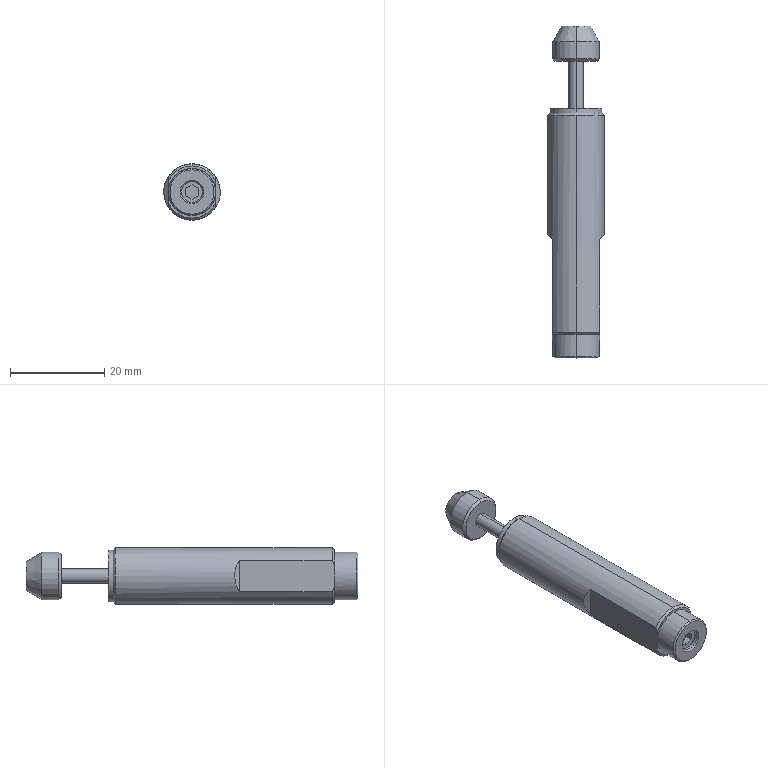Part | SolidWorks | features BaseBody 1 | 1 solid | 46 faces | box 12 x 70.5 x 12 mm | volume 6151 mm3 | plane 19 | cone 15 | cylinder 12 | commonest cylinder face diameters 10 x4 3 x2 4.459 x2 11 x2 12 x2
STEP:
#1=CARTESIAN_POINT('',(6.,51.54,0.));
#2=VERTEX_POINT('',#1);
#3=CARTESIAN_POINT('',(0.,51.54,6.));
#4=VERTEX_POINT('',#3);
#5=CARTESIAN_POINT('',(0.,51.54,0.));
#6=DIRECTION('',(0.,-1.,0.));
#7=DIRECTION('',(0.,0.,-1.));
#8=AXIS2_PLACEMENT_3D('',#5,#6,#7);
#9=CIRCLE('',#8,6.);
#10=EDGE_CURVE('',#2,#4,#9,.T.);
#11=ORIENTED_EDGE('',*,*,#10,.T.);
#12=CARTESIAN_POINT('',(0.,5.46,6.));
#13=VERTEX_POINT('',#12);
#14=CARTESIAN_POINT('',(0.,0.,6.));
#15=DIRECTION('',(0.,-1.,0.));
#16=VECTOR('',#15,1000.);
#17=LINE('',#14,#16);
#18=EDGE_CURVE('',#4,#13,#17,.T.);
#19=ORIENTED_EDGE('',*,*,#18,.T.);
#20=CARTESIAN_POINT('',(5.,5.46,3.317));
#21=VERTEX_POINT('',#20);
#22=CARTESIAN_POINT('',(0.,5.46,0.));
#23=DIRECTION('',(0.,1.,0.));
#24=DIRECTION('',(0.,0.,-1.));
#25=AXIS2_PLACEMENT_3D('',#22,#23,#24);
#26=CIRCLE('',#25,6.);
#27=EDGE_CURVE('',#13,#21,#26,.T.);
#28=ORIENTED_EDGE('',*,*,#27,.T.);
#29=CARTESIAN_POINT('',(5.,25.177,3.317));
#30=VERTEX_POINT('',#29);
#31=CARTESIAN_POINT('',(5.,0.,3.317));
#32=DIRECTION('',(0.,1.,0.));
#33=VECTOR('',#32,1000.);
#34=LINE('',#31,#33);
#35=EDGE_CURVE('',#21,#30,#34,.T.);
#36=ORIENTED_EDGE('',*,*,#35,.T.);
#37=CARTESIAN_POINT('',(5.,25.177,-3.317));
#38=VERTEX_POINT('',#37);
#39=CARTESIAN_POINT('',(5.,25.177,3.317));
#40=CARTESIAN_POINT('',(6.375,26.552,1.244));
#41=CARTESIAN_POINT('',(6.375,26.552,-1.244));
#42=CARTESIAN_POINT('',(5.,25.177,-3.317));
#43=(BOUNDED_CURVE()B_SPLINE_CURVE(3,(#39,#40,#41,#42),.UNSPECIFIED.,.F.,.F.)B_SPLINE_CURVE_WITH_KNOTS((4,4),(2.556,3.727),.UNSPECIFIED.)CURVE()GEOMETRIC_REPRESENTATION_ITEM()RATIONAL_B_SPLINE_CURVE((1.,0.8889,0.8889,1.))REPRESENTATION_ITEM(''));
#44=EDGE_CURVE('',#30,#38,#43,.T.);
#45=ORIENTED_EDGE('',*,*,#44,.T.);
#46=CARTESIAN_POINT('',(5.,5.46,-3.317));
#47=VERTEX_POINT('',#46);
#48=CARTESIAN_POINT('',(5.,0.,-3.317));
#49=DIRECTION('',(0.,-1.,0.));
#50=VECTOR('',#49,1000.);
#51=LINE('',#48,#50);
#52=EDGE_CURVE('',#38,#47,#51,.T.);
#53=ORIENTED_EDGE('',*,*,#52,.T.);
#54=CARTESIAN_POINT('',(0.,5.46,-6.));
#55=VERTEX_POINT('',#54);
#56=CARTESIAN_POINT('',(0.,5.46,0.));
#57=DIRECTION('',(0.,1.,0.));
#58=DIRECTION('',(0.,0.,-1.));
#59=AXIS2_PLACEMENT_3D('',#56,#57,#58);
#60=CIRCLE('',#59,6.);
#61=EDGE_CURVE('',#47,#55,#60,.T.);
#62=ORIENTED_EDGE('',*,*,#61,.T.);
#63=CARTESIAN_POINT('',(0.,51.54,-6.));
#64=VERTEX_POINT('',#63);
#65=CARTESIAN_POINT('',(0.,0.,-6.));
#66=DIRECTION('',(0.,-1.,0.));
#67=VECTOR('',#66,1000.);
#68=LINE('',#65,#67);
#69=EDGE_CURVE('',#64,#55,#68,.T.);
#70=ORIENTED_EDGE('',*,*,#69,.F.);
#71=CARTESIAN_POINT('',(0.,51.54,0.));
#72=DIRECTION('',(0.,-1.,0.));
#73=DIRECTION('',(0.,0.,-1.));
#74=AXIS2_PLACEMENT_3D('',#71,#72,#73);
#75=CIRCLE('',#74,6.);
#76=EDGE_CURVE('',#64,#2,#75,.T.);
#77=ORIENTED_EDGE('',*,*,#76,.T.);
#78=EDGE_LOOP('',(#11,#19,#28,#36,#45,#53,#62,#70,#77));
#79=FACE_OUTER_BOUND('',#78,.T.);
#80=CARTESIAN_POINT('',(0.,0.,0.));
#81=DIRECTION('',(0.,-1.,0.));
#82=DIRECTION('',(0.,0.,-1.));
#83=AXIS2_PLACEMENT_3D('',#80,#81,#82);
#84=CYLINDRICAL_SURFACE('',#83,6.);
#85=ADVANCED_FACE('',(#79),#84,.T.);
#86=CARTESIAN_POINT('',(5.54,52.,0.));
#87=VERTEX_POINT('',#86);
#88=CARTESIAN_POINT('',(-5.54,52.,0.));
#89=VERTEX_POINT('',#88);
#90=CARTESIAN_POINT('',(0.,52.,0.));
#91=DIRECTION('',(0.,-1.,0.));
#92=DIRECTION('',(1.,0.,0.));
#93=AXIS2_PLACEMENT_3D('',#90,#91,#92);
#94=CIRCLE('',#93,5.54);
#95=EDGE_CURVE('',#87,#89,#94,.T.);
#96=ORIENTED_EDGE('',*,*,#95,.T.);
#97=CARTESIAN_POINT('',(-6.,51.54,0.));
#98=VERTEX_POINT('',#97);
#99=CARTESIAN_POINT('',(-6.,51.54,0.));
#100=DIRECTION('',(-0.7071,-0.7071,0.));
#101=VECTOR('',#100,1000.);
#102=LINE('',#99,#101);
#103=EDGE_CURVE('',#89,#98,#102,.T.);
#104=ORIENTED_EDGE('',*,*,#103,.T.);
#105=CARTESIAN_POINT('',(0.,51.54,0.));
#106=DIRECTION('',(0.,-1.,0.));
#107=DIRECTION('',(0.,0.,-1.));
#108=AXIS2_PLACEMENT_3D('',#105,#106,#107);
#109=CIRCLE('',#108,6.);
#110=EDGE_CURVE('',#4,#98,#109,.T.);
#111=ORIENTED_EDGE('',*,*,#110,.F.);
#112=ORIENTED_EDGE('',*,*,#10,.F.);
#113=CARTESIAN_POINT('',(6.,51.54,0.));
#114=DIRECTION('',(0.7071,-0.7071,0.));
#115=VECTOR('',#114,1000.);
#116=LINE('',#113,#115);
#117=EDGE_CURVE('',#87,#2,#116,.T.);
#118=ORIENTED_EDGE('',*,*,#117,.F.);
#119=EDGE_LOOP('',(#96,#104,#111,#112,#118));
#120=FACE_OUTER_BOUND('',#119,.T.);
#121=CARTESIAN_POINT('',(0.,51.54,0.));
#122=DIRECTION('',(0.,-1.,0.));
#123=DIRECTION('',(1.,0.,0.));
#124=AXIS2_PLACEMENT_3D('',#121,#122,#123);
#125=CONICAL_SURFACE('',#124,6.,0.7854);
#126=ADVANCED_FACE('',(#120),#125,.T.);
#127=CARTESIAN_POINT('',(-5.,5.,2.386));
#128=VERTEX_POINT('',#127);
#129=CARTESIAN_POINT('',(0.,5.,5.54));
#130=VERTEX_POINT('',#129);
#131=CARTESIAN_POINT('',(0.,5.,0.));
#132=DIRECTION('',(0.,1.,0.));
#133=DIRECTION('',(0.,0.,1.));
#134=AXIS2_PLACEMENT_3D('',#131,#132,#133);
#135=CIRCLE('',#134,5.54);
#136=EDGE_CURVE('',#128,#130,#135,.T.);
#137=ORIENTED_EDGE('',*,*,#136,.T.);
#138=CARTESIAN_POINT('',(0.,5.46,6.));
#139=DIRECTION('',(0.,0.7071,0.7071));
#140=VECTOR('',#139,1000.);
#141=LINE('',#138,#140);
#142=EDGE_CURVE('',#130,#13,#141,.T.);
#143=ORIENTED_EDGE('',*,*,#142,.T.);
#144=CARTESIAN_POINT('',(-5.,5.46,3.317));
#145=VERTEX_POINT('',#144);
#146=CARTESIAN_POINT('',(0.,5.46,0.));
#147=DIRECTION('',(0.,1.,0.));
#148=DIRECTION('',(0.,0.,-1.));
#149=AXIS2_PLACEMENT_3D('',#146,#147,#148);
#150=CIRCLE('',#149,6.);
#151=EDGE_CURVE('',#145,#13,#150,.T.);
#152=ORIENTED_EDGE('',*,*,#151,.F.);
#153=CARTESIAN_POINT('',(-5.,5.46,3.317));
#154=CARTESIAN_POINT('',(-5.,5.292,3.013));
#155=CARTESIAN_POINT('',(-5.,5.137,2.704));
#156=CARTESIAN_POINT('',(-5.,5.,2.386));
#157=B_SPLINE_CURVE_WITH_KNOTS('',3,(#153,#154,#155,#156),.UNSPECIFIED.,.F.,.F.,(4,4),(0.,0.001038),.UNSPECIFIED.);
#158=EDGE_CURVE('',#145,#128,#157,.T.);
#159=ORIENTED_EDGE('',*,*,#158,.T.);
#160=EDGE_LOOP('',(#137,#143,#152,#159));
#161=FACE_OUTER_BOUND('',#160,.T.);
#162=CARTESIAN_POINT('',(0.,5.46,0.));
#163=DIRECTION('',(0.,1.,0.));
#164=DIRECTION('',(0.,0.,1.));
#165=AXIS2_PLACEMENT_3D('',#162,#163,#164);
#166=CONICAL_SURFACE('',#165,6.,0.7854);
#167=ADVANCED_FACE('',(#161),#166,.T.);
#168=CARTESIAN_POINT('',(0.,53.,-5.5));
#169=VERTEX_POINT('',#168);
#170=CARTESIAN_POINT('',(0.,53.,5.5));
#171=VERTEX_POINT('',#170);
#172=CARTESIAN_POINT('',(0.,53.,0.));
#173=DIRECTION('',(0.,-1.,0.));
#174=DIRECTION('',(0.,0.,-1.));
#175=AXIS2_PLACEMENT_3D('',#172,#173,#174);
#176=CIRCLE('',#175,5.5);
#177=EDGE_CURVE('',#169,#171,#176,.T.);
#178=ORIENTED_EDGE('',*,*,#177,.T.);
#179=CARTESIAN_POINT('',(0.,52.,5.5));
#180=VERTEX_POINT('',#179);
#181=CARTESIAN_POINT('',(0.,0.,5.5));
#182=DIRECTION('',(0.,-1.,0.));
#183=VECTOR('',#182,1000.);
#184=LINE('',#181,#183);
#185=EDGE_CURVE('',#171,#180,#184,.T.);
#186=ORIENTED_EDGE('',*,*,#185,.T.);
#187=CARTESIAN_POINT('',(0.,52.,-5.5));
#188=VERTEX_POINT('',#187);
#189=CARTESIAN_POINT('',(0.,52.,0.));
#190=DIRECTION('',(0.,1.,0.));
#191=DIRECTION('',(0.,0.,-1.));
#192=AXIS2_PLACEMENT_3D('',#189,#190,#191);
#193=CIRCLE('',#192,5.5);
#194=EDGE_CURVE('',#180,#188,#193,.T.);
#195=ORIENTED_EDGE('',*,*,#194,.T.);
#196=CARTESIAN_POINT('',(0.,0.,-5.5));
#197=DIRECTION('',(0.,-1.,0.));
#198=VECTOR('',#197,1000.);
#199=LINE('',#196,#198);
#200=EDGE_CURVE('',#169,#188,#199,.T.);
#201=ORIENTED_EDGE('',*,*,#200,.F.);
#202=EDGE_LOOP('',(#178,#186,#195,#201));
#203=FACE_OUTER_BOUND('',#202,.T.);
#204=CARTESIAN_POINT('',(0.,0.,0.));
#205=DIRECTION('',(0.,-1.,0.));
#206=DIRECTION('',(0.,0.,-1.));
#207=AXIS2_PLACEMENT_3D('',#204,#205,#206);
#208=CYLINDRICAL_SURFACE('',#207,5.5);
#209=ADVANCED_FACE('',(#203),#208,.T.);
#210=CARTESIAN_POINT('',(5.,5.,0.));
#211=VERTEX_POINT('',#210);
#212=CARTESIAN_POINT('',(0.,5.,5.));
#213=VERTEX_POINT('',#212);
#214=CARTESIAN_POINT('',(0.,5.,0.));
#215=DIRECTION('',(0.,-1.,0.));
#216=DIRECTION('',(0.,0.,-1.));
#217=AXIS2_PLACEMENT_3D('',#214,#215,#216);
#218=CIRCLE('',#217,5.);
#219=EDGE_CURVE('',#211,#213,#218,.T.);
#220=ORIENTED_EDGE('',*,*,#219,.T.);
#221=CARTESIAN_POINT('',(0.,0.3,5.));
#222=VERTEX_POINT('',#221);
#223=CARTESIAN_POINT('',(0.,0.,5.));
#224=DIRECTION('',(0.,-1.,0.));
#225=VECTOR('',#224,1000.);
#226=LINE('',#223,#225);
#227=EDGE_CURVE('',#213,#222,#226,.T.);
#228=ORIENTED_EDGE('',*,*,#227,.T.);
#229=CARTESIAN_POINT('',(0.,0.3,-5.));
#230=VERTEX_POINT('',#229);
#231=CARTESIAN_POINT('',(0.,0.3,0.));
#232=DIRECTION('',(0.,1.,0.));
#233=DIRECTION('',(0.,0.,-1.));
#234=AXIS2_PLACEMENT_3D('',#231,#232,#233);
#235=CIRCLE('',#234,5.);
#236=EDGE_CURVE('',#222,#230,#235,.T.);
#237=ORIENTED_EDGE('',*,*,#236,.T.);
#238=CARTESIAN_POINT('',(0.,5.,-5.));
#239=VERTEX_POINT('',#238);
#240=CARTESIAN_POINT('',(0.,0.,-5.));
#241=DIRECTION('',(0.,-1.,0.));
#242=VECTOR('',#241,1000.);
#243=LINE('',#240,#242);
#244=EDGE_CURVE('',#239,#230,#243,.T.);
#245=ORIENTED_EDGE('',*,*,#244,.F.);
#246=CARTESIAN_POINT('',(0.,5.,0.));
#247=DIRECTION('',(0.,-1.,0.));
#248=DIRECTION('',(0.,0.,-1.));
#249=AXIS2_PLACEMENT_3D('',#246,#247,#248);
#250=CIRCLE('',#249,5.);
#251=EDGE_CURVE('',#239,#211,#250,.T.);
#252=ORIENTED_EDGE('',*,*,#251,.T.);
#253=EDGE_LOOP('',(#220,#228,#237,#245,#252));
#254=FACE_OUTER_BOUND('',#253,.T.);
#255=CARTESIAN_POINT('',(0.,0.,0.));
#256=DIRECTION('',(0.,-1.,0.));
#257=DIRECTION('',(0.,0.,-1.));
#258=AXIS2_PLACEMENT_3D('',#255,#256,#257);
#259=CYLINDRICAL_SURFACE('',#258,5.);
#260=ADVANCED_FACE('',(#254),#259,.T.);
#261=CARTESIAN_POINT('',(0.,0.,4.7));
#262=VERTEX_POINT('',#261);
#263=CARTESIAN_POINT('',(0.,0.,-4.7));
#264=VERTEX_POINT('',#263);
#265=CARTESIAN_POINT('',(0.,0.,0.));
#266=DIRECTION('',(0.,1.,0.));
#267=DIRECTION('',(0.,0.,1.));
#268=AXIS2_PLACEMENT_3D('',#265,#266,#267);
#269=CIRCLE('',#268,4.7);
#270=EDGE_CURVE('',#262,#264,#269,.T.);
#271=ORIENTED_EDGE('',*,*,#270,.T.);
#272=CARTESIAN_POINT('',(0.,0.3,-5.));
#273=DIRECTION('',(0.,0.7071,-0.7071));
#274=VECTOR('',#273,1000.);
#275=LINE('',#272,#274);
#276=EDGE_CURVE('',#264,#230,#275,.T.);
#277=ORIENTED_EDGE('',*,*,#276,.T.);
#278=ORIENTED_EDGE('',*,*,#236,.F.);
#279=CARTESIAN_POINT('',(0.,0.3,5.));
#280=DIRECTION('',(0.,0.7071,0.7071));
#281=VECTOR('',#280,1000.);
#282=LINE('',#279,#281);
#283=EDGE_CURVE('',#262,#222,#282,.T.);
#284=ORIENTED_EDGE('',*,*,#283,.F.);
#285=EDGE_LOOP('',(#271,#277,#278,#284));
#286=FACE_OUTER_BOUND('',#285,.T.);
#287=CARTESIAN_POINT('',(0.,0.3,0.));
#288=DIRECTION('',(0.,1.,0.));
#289=DIRECTION('',(0.,0.,1.));
#290=AXIS2_PLACEMENT_3D('',#287,#288,#289);
#291=CONICAL_SURFACE('',#290,5.,0.7854);
#292=ADVANCED_FACE('',(#286),#291,.T.);
#293=CARTESIAN_POINT('',(0.,63.,-1.5));
#294=VERTEX_POINT('',#293);
#295=CARTESIAN_POINT('',(0.,63.,1.5));
#296=VERTEX_POINT('',#295);
#297=CARTESIAN_POINT('',(0.,63.,0.));
#298=DIRECTION('',(0.,-1.,0.));
#299=DIRECTION('',(0.,0.,-1.));
#300=AXIS2_PLACEMENT_3D('',#297,#298,#299);
#301=CIRCLE('',#300,1.5);
#302=EDGE_CURVE('',#294,#296,#301,.T.);
#303=ORIENTED_EDGE('',*,*,#302,.T.);
#304=CARTESIAN_POINT('',(0.,53.,1.5));
#305=VERTEX_POINT('',#304);
#306=CARTESIAN_POINT('',(0.,0.,1.5));
#307=DIRECTION('',(0.,-1.,0.));
#308=VECTOR('',#307,1000.);
#309=LINE('',#306,#308);
#310=EDGE_CURVE('',#296,#305,#309,.T.);
#311=ORIENTED_EDGE('',*,*,#310,.T.);
#312=CARTESIAN_POINT('',(0.,53.,-1.5));
#313=VERTEX_POINT('',#312);
#314=CARTESIAN_POINT('',(0.,53.,0.));
#315=DIRECTION('',(0.,1.,0.));
#316=DIRECTION('',(0.,0.,-1.));
#317=AXIS2_PLACEMENT_3D('',#314,#315,#316);
#318=CIRCLE('',#317,1.5);
#319=EDGE_CURVE('',#305,#313,#318,.T.);
#320=ORIENTED_EDGE('',*,*,#319,.T.);
#321=CARTESIAN_POINT('',(0.,0.,-1.5));
#322=DIRECTION('',(0.,-1.,0.));
#323=VECTOR('',#322,1000.);
#324=LINE('',#321,#323);
#325=EDGE_CURVE('',#294,#313,#324,.T.);
#326=ORIENTED_EDGE('',*,*,#325,.F.);
#327=EDGE_LOOP('',(#303,#311,#320,#326));
#328=FACE_OUTER_BOUND('',#327,.T.);
#329=CARTESIAN_POINT('',(0.,0.,0.));
#330=DIRECTION('',(0.,-1.,0.));
#331=DIRECTION('',(0.,0.,-1.));
#332=AXIS2_PLACEMENT_3D('',#329,#330,#331);
#333=CYLINDRICAL_SURFACE('',#332,1.5);
#334=ADVANCED_FACE('',(#328),#333,.T.);
#335=CARTESIAN_POINT('',(0.,0.2705,2.229));
#336=VERTEX_POINT('',#335);
#337=CARTESIAN_POINT('',(0.,0.2705,-2.229));
#338=VERTEX_POINT('',#337);
#339=CARTESIAN_POINT('',(0.,0.2705,0.));
#340=DIRECTION('',(0.,-1.,0.));
#341=DIRECTION('',(0.,0.,-1.));
#342=AXIS2_PLACEMENT_3D('',#339,#340,#341);
#343=CIRCLE('',#342,2.229);
#344=EDGE_CURVE('',#336,#338,#343,.T.);
#345=ORIENTED_EDGE('',*,*,#344,.F.);
#346=CARTESIAN_POINT('',(0.,0.,2.5));
#347=VERTEX_POINT('',#346);
#348=CARTESIAN_POINT('',(0.,0.,2.5));
#349=DIRECTION('',(0.,-0.7071,0.7071));
#350=VECTOR('',#349,1000.);
#351=LINE('',#348,#350);
#352=EDGE_CURVE('',#336,#347,#351,.T.);
#353=ORIENTED_EDGE('',*,*,#352,.T.);
#354=CARTESIAN_POINT('',(0.,0.,-2.5));
#355=VERTEX_POINT('',#354);
#356=CARTESIAN_POINT('',(0.,0.,0.));
#357=DIRECTION('',(0.,-1.,0.));
#358=DIRECTION('',(0.,0.,-1.));
#359=AXIS2_PLACEMENT_3D('',#356,#357,#358);
#360=CIRCLE('',#359,2.5);
#361=EDGE_CURVE('',#347,#355,#360,.T.);
#362=ORIENTED_EDGE('',*,*,#361,.T.);
#363=CARTESIAN_POINT('',(0.,0.,-2.5));
#364=DIRECTION('',(0.,-0.7071,-0.7071));
#365=VECTOR('',#364,1000.);
#366=LINE('',#363,#365);
#367=EDGE_CURVE('',#338,#355,#366,.T.);
#368=ORIENTED_EDGE('',*,*,#367,.F.);
#369=EDGE_LOOP('',(#345,#353,#362,#368));
#370=FACE_OUTER_BOUND('',#369,.T.);
#371=CARTESIAN_POINT('',(0.,0.,0.));
#372=DIRECTION('',(0.,-1.,0.));
#373=DIRECTION('',(0.,0.,-1.));
#374=AXIS2_PLACEMENT_3D('',#371,#372,#373);
#375=CONICAL_SURFACE('',#374,2.5,0.7854);
#376=ADVANCED_FACE('',(#370),#375,.F.);
#377=CARTESIAN_POINT('',(0.,63.,4.5));
#378=VERTEX_POINT('',#377);
#379=CARTESIAN_POINT('',(0.,63.,-4.5));
#380=VERTEX_POINT('',#379);
#381=CARTESIAN_POINT('',(0.,63.,0.));
#382=DIRECTION('',(0.,1.,0.));
#383=DIRECTION('',(0.,0.,1.));
#384=AXIS2_PLACEMENT_3D('',#381,#382,#383);
#385=CIRCLE('',#384,4.5);
#386=EDGE_CURVE('',#378,#380,#385,.T.);
#387=ORIENTED_EDGE('',*,*,#386,.T.);
#388=CARTESIAN_POINT('',(0.,63.5,-5.));
#389=VERTEX_POINT('',#388);
#390=CARTESIAN_POINT('',(0.,63.5,-5.));
#391=DIRECTION('',(0.,0.7071,-0.7071));
#392=VECTOR('',#391,1000.);
#393=LINE('',#390,#392);
#394=EDGE_CURVE('',#380,#389,#393,.T.);
#395=ORIENTED_EDGE('',*,*,#394,.T.);
#396=CARTESIAN_POINT('',(0.,63.5,5.));
#397=VERTEX_POINT('',#396);
#398=CARTESIAN_POINT('',(0.,63.5,0.));
#399=DIRECTION('',(0.,-1.,0.));
#400=DIRECTION('',(0.,0.,1.));
#401=AXIS2_PLACEMENT_3D('',#398,#399,#400);
#402=CIRCLE('',#401,5.);
#403=EDGE_CURVE('',#389,#397,#402,.T.);
#404=ORIENTED_EDGE('',*,*,#403,.T.);
#405=CARTESIAN_POINT('',(0.,63.5,5.));
#406=DIRECTION('',(0.,0.7071,0.7071));
#407=VECTOR('',#406,1000.);
#408=LINE('',#405,#407);
#409=EDGE_CURVE('',#378,#397,#408,.T.);
#410=ORIENTED_EDGE('',*,*,#409,.F.);
#411=EDGE_LOOP('',(#387,#395,#404,#410));
#412=FACE_OUTER_BOUND('',#411,.T.);
#413=CARTESIAN_POINT('',(0.,63.5,0.));
#414=DIRECTION('',(0.,1.,0.));
#415=DIRECTION('',(0.,0.,1.));
#416=AXIS2_PLACEMENT_3D('',#413,#414,#415);
#417=CONICAL_SURFACE('',#416,5.,0.7854);
#418=ADVANCED_FACE('',(#412),#417,.T.);
#419=CARTESIAN_POINT('',(0.,0.9295,2.229));
#420=VERTEX_POINT('',#419);
#421=CARTESIAN_POINT('',(0.,0.9295,-2.229));
#422=VERTEX_POINT('',#421);
#423=CARTESIAN_POINT('',(0.,0.9295,0.));
#424=DIRECTION('',(0.,-1.,0.));
#425=DIRECTION('',(0.,0.,-1.));
#426=AXIS2_PLACEMENT_3D('',#423,#424,#425);
#427=CIRCLE('',#426,2.229);
#428=EDGE_CURVE('',#420,#422,#427,.T.);
#429=ORIENTED_EDGE('',*,*,#428,.F.);
#430=CARTESIAN_POINT('',(0.,0.,2.229));
#431=DIRECTION('',(0.,-1.,0.));
#432=VECTOR('',#431,1000.);
#433=LINE('',#430,#432);
#434=EDGE_CURVE('',#420,#336,#433,.T.);
#435=ORIENTED_EDGE('',*,*,#434,.T.);
#436=ORIENTED_EDGE('',*,*,#344,.T.);
#437=CARTESIAN_POINT('',(0.,0.,-2.229));
#438=DIRECTION('',(0.,-1.,0.));
#439=VECTOR('',#438,1000.);
#440=LINE('',#437,#439);
#441=EDGE_CURVE('',#422,#338,#440,.T.);
#442=ORIENTED_EDGE('',*,*,#441,.F.);
#443=EDGE_LOOP('',(#429,#435,#436,#442));
#444=FACE_OUTER_BOUND('',#443,.T.);
#445=CARTESIAN_POINT('',(0.,0.,0.));
#446=DIRECTION('',(0.,-1.,0.));
#447=DIRECTION('',(0.,0.,-1.));
#448=AXIS2_PLACEMENT_3D('',#445,#446,#447);
#449=CYLINDRICAL_SURFACE('',#448,2.229);
#450=ADVANCED_FACE('',(#444),#449,.F.);
#451=CARTESIAN_POINT('',(0.,67.167,-5.));
#452=VERTEX_POINT('',#451);
#453=CARTESIAN_POINT('',(0.,67.167,5.));
#454=VERTEX_POINT('',#453);
#455=CARTESIAN_POINT('',(0.,67.167,0.));
#456=DIRECTION('',(0.,-1.,0.));
#457=DIRECTION('',(0.,0.,-1.));
#458=AXIS2_PLACEMENT_3D('',#455,#456,#457);
#459=CIRCLE('',#458,5.);
#460=EDGE_CURVE('',#452,#454,#459,.T.);
#461=ORIENTED_EDGE('',*,*,#460,.T.);
#462=CARTESIAN_POINT('',(0.,0.,5.));
#463=DIRECTION('',(0.,-1.,0.));
#464=VECTOR('',#463,1000.);
#465=LINE('',#462,#464);
#466=EDGE_CURVE('',#454,#397,#465,.T.);
#467=ORIENTED_EDGE('',*,*,#466,.T.);
#468=ORIENTED_EDGE('',*,*,#403,.F.);
#469=CARTESIAN_POINT('',(0.,0.,-5.));
#470=DIRECTION('',(0.,-1.,0.));
#471=VECTOR('',#470,1000.);
#472=LINE('',#469,#471);
#473=EDGE_CURVE('',#452,#389,#472,.T.);
#474=ORIENTED_EDGE('',*,*,#473,.F.);
#475=EDGE_LOOP('',(#461,#467,#468,#474));
#476=FACE_OUTER_BOUND('',#475,.T.);
#477=CARTESIAN_POINT('',(0.,0.,0.));
#478=DIRECTION('',(0.,-1.,0.));
#479=DIRECTION('',(0.,0.,-1.));
#480=AXIS2_PLACEMENT_3D('',#477,#478,#479);
#481=CYLINDRICAL_SURFACE('',#480,5.);
#482=ADVANCED_FACE('',(#476),#481,.T.);
#483=ORIENTED_EDGE('',*,*,#428,.T.);
#484=CARTESIAN_POINT('',(0.,1.2,-2.5));
#485=VERTEX_POINT('',#484);
#486=CARTESIAN_POINT('',(0.,1.2,-2.5));
#487=DIRECTION('',(0.,0.7071,-0.7071));
#488=VECTOR('',#487,1000.);
#489=LINE('',#486,#488);
#490=EDGE_CURVE('',#422,#485,#489,.T.);
#491=ORIENTED_EDGE('',*,*,#490,.T.);
#492=CARTESIAN_POINT('',(0.,1.2,2.5));
#493=VERTEX_POINT('',#492);
#494=CARTESIAN_POINT('',(0.,1.2,0.));
#495=DIRECTION('',(0.,-1.,0.));
#496=DIRECTION('',(0.,0.,1.));
#497=AXIS2_PLACEMENT_3D('',#494,#495,#496);
#498=CIRCLE('',#497,2.5);
#499=EDGE_CURVE('',#493,#485,#498,.T.);
#500=ORIENTED_EDGE('',*,*,#499,.F.);
#501=CARTESIAN_POINT('',(0.,1.2,2.5));
#502=DIRECTION('',(0.,0.7071,0.7071));
#503=VECTOR('',#502,1000.);
#504=LINE('',#501,#503);
#505=EDGE_CURVE('',#420,#493,#504,.T.);
#506=ORIENTED_EDGE('',*,*,#505,.F.);
#507=EDGE_LOOP('',(#483,#491,#500,#506));
#508=FACE_OUTER_BOUND('',#507,.T.);
#509=CARTESIAN_POINT('',(0.,1.2,0.));
#510=DIRECTION('',(0.,1.,0.));
#511=DIRECTION('',(0.,0.,1.));
#512=AXIS2_PLACEMENT_3D('',#509,#510,#511);
#513=CONICAL_SURFACE('',#512,2.5,0.7854);
#514=ADVANCED_FACE('',(#508),#513,.F.);
#515=CARTESIAN_POINT('',(0.,70.5,-3.075));
#516=VERTEX_POINT('',#515);
#517=CARTESIAN_POINT('',(0.,70.5,3.075));
#518=VERTEX_POINT('',#517);
#519=CARTESIAN_POINT('',(0.,70.5,0.));
#520=DIRECTION('',(0.,-1.,0.));
#521=DIRECTION('',(0.,0.,-1.));
#522=AXIS2_PLACEMENT_3D('',#519,#520,#521);
#523=CIRCLE('',#522,3.075);
#524=EDGE_CURVE('',#516,#518,#523,.T.);
#525=ORIENTED_EDGE('',*,*,#524,.T.);
#526=CARTESIAN_POINT('',(0.,67.167,5.));
#527=DIRECTION('',(0.,-0.866,0.5));
#528=VECTOR('',#527,1000.);
#529=LINE('',#526,#528);
#530=EDGE_CURVE('',#518,#454,#529,.T.);
#531=ORIENTED_EDGE('',*,*,#530,.T.);
#532=ORIENTED_EDGE('',*,*,#460,.F.);
#533=CARTESIAN_POINT('',(0.,67.167,-5.));
#534=DIRECTION('',(0.,-0.866,-0.5));
#535=VECTOR('',#534,1000.);
#536=LINE('',#533,#535);
#537=EDGE_CURVE('',#516,#452,#536,.T.);
#538=ORIENTED_EDGE('',*,*,#537,.F.);
#539=EDGE_LOOP('',(#525,#531,#532,#538));
#540=FACE_OUTER_BOUND('',#539,.T.);
#541=CARTESIAN_POINT('',(0.,67.167,0.));
#542=DIRECTION('',(0.,-1.,0.));
#543=DIRECTION('',(0.,0.,-1.));
#544=AXIS2_PLACEMENT_3D('',#541,#542,#543);
#545=CONICAL_SURFACE('',#544,5.,0.5236);
#546=ADVANCED_FACE('',(#540),#545,.T.);
#547=ORIENTED_EDGE('',*,*,#18,.F.);
#548=ORIENTED_EDGE('',*,*,#110,.T.);
#549=CARTESIAN_POINT('',(0.,51.54,0.));
#550=DIRECTION('',(0.,-1.,0.));
#551=DIRECTION('',(0.,0.,-1.));
#552=AXIS2_PLACEMENT_3D('',#549,#550,#551);
#553=CIRCLE('',#552,6.);
#554=EDGE_CURVE('',#98,#64,#553,.T.);
#555=ORIENTED_EDGE('',*,*,#554,.T.);
#556=ORIENTED_EDGE('',*,*,#69,.T.);
#557=CARTESIAN_POINT('',(-5.,5.46,-3.317));
#558=VERTEX_POINT('',#557);
#559=CARTESIAN_POINT('',(0.,5.46,0.));
#560=DIRECTION('',(0.,1.,0.));
#561=DIRECTION('',(0.,0.,-1.));
#562=AXIS2_PLACEMENT_3D('',#559,#560,#561);
#563=CIRCLE('',#562,6.);
#564=EDGE_CURVE('',#55,#558,#563,.T.);
#565=ORIENTED_EDGE('',*,*,#564,.T.);
#566=CARTESIAN_POINT('',(-5.,25.177,-3.317));
#567=VERTEX_POINT('',#566);
#568=CARTESIAN_POINT('',(-5.,0.,-3.317));
#569=DIRECTION('',(0.,1.,0.));
#570=VECTOR('',#569,1000.);
#571=LINE('',#568,#570);
#572=EDGE_CURVE('',#558,#567,#571,.T.);
#573=ORIENTED_EDGE('',*,*,#572,.T.);
#574=CARTESIAN_POINT('',(-5.,25.177,3.317));
#575=VERTEX_POINT('',#574);
#576=CARTESIAN_POINT('',(-5.,25.177,-3.317));
#577=CARTESIAN_POINT('',(-6.375,26.552,-1.244));
#578=CARTESIAN_POINT('',(-6.375,26.552,1.244));
#579=CARTESIAN_POINT('',(-5.,25.177,3.317));
#580=(BOUNDED_CURVE()B_SPLINE_CURVE(3,(#576,#577,#578,#579),.UNSPECIFIED.,.F.,.F.)B_SPLINE_CURVE_WITH_KNOTS((4,4),(2.556,3.727),.UNSPECIFIED.)CURVE()GEOMETRIC_REPRESENTATION_ITEM()RATIONAL_B_SPLINE_CURVE((1.,0.8889,0.8889,1.))REPRESENTATION_ITEM(''));
#581=EDGE_CURVE('',#567,#575,#580,.T.);
#582=ORIENTED_EDGE('',*,*,#581,.T.);
#583=CARTESIAN_POINT('',(-5.,0.,3.317));
#584=DIRECTION('',(0.,-1.,0.));
#585=VECTOR('',#584,1000.);
#586=LINE('',#583,#585);
#587=EDGE_CURVE('',#575,#145,#586,.T.);
#588=ORIENTED_EDGE('',*,*,#587,.T.);
#589=ORIENTED_EDGE('',*,*,#151,.T.);
#590=EDGE_LOOP('',(#547,#548,#555,#556,#565,#573,#582,#588,#589));
#591=FACE_OUTER_BOUND('',#590,.T.);
#592=CARTESIAN_POINT('',(0.,0.,0.));
#593=DIRECTION('',(0.,-1.,0.));
#594=DIRECTION('',(0.,0.,-1.));
#595=AXIS2_PLACEMENT_3D('',#592,#593,#594);
#596=CYLINDRICAL_SURFACE('',#595,6.);
#597=ADVANCED_FACE('',(#591),#596,.T.);
#598=ORIENTED_EDGE('',*,*,#103,.F.);
#599=CARTESIAN_POINT('',(0.,52.,0.));
#600=DIRECTION('',(0.,-1.,0.));
#601=DIRECTION('',(1.,0.,0.));
#602=AXIS2_PLACEMENT_3D('',#599,#600,#601);
#603=CIRCLE('',#602,5.54);
#604=EDGE_CURVE('',#89,#87,#603,.T.);
#605=ORIENTED_EDGE('',*,*,#604,.T.);
#606=ORIENTED_EDGE('',*,*,#117,.T.);
#607=ORIENTED_EDGE('',*,*,#76,.F.);
#608=ORIENTED_EDGE('',*,*,#554,.F.);
#609=EDGE_LOOP('',(#598,#605,#606,#607,#608));
#610=FACE_OUTER_BOUND('',#609,.T.);
#611=CARTESIAN_POINT('',(0.,51.54,0.));
#612=DIRECTION('',(0.,-1.,0.));
#613=DIRECTION('',(1.,0.,0.));
#614=AXIS2_PLACEMENT_3D('',#611,#612,#613);
#615=CONICAL_SURFACE('',#614,6.,0.7854);
#616=ADVANCED_FACE('',(#610),#615,.T.);
#617=ORIENTED_EDGE('',*,*,#142,.F.);
#618=CARTESIAN_POINT('',(5.,5.,2.386));
#619=VERTEX_POINT('',#618);
#620=CARTESIAN_POINT('',(0.,5.,0.));
#621=DIRECTION('',(0.,1.,0.));
#622=DIRECTION('',(0.,0.,1.));
#623=AXIS2_PLACEMENT_3D('',#620,#621,#622);
#624=CIRCLE('',#623,5.54);
#625=EDGE_CURVE('',#130,#619,#624,.T.);
#626=ORIENTED_EDGE('',*,*,#625,.T.);
#627=CARTESIAN_POINT('',(5.,5.,2.386));
#628=CARTESIAN_POINT('',(5.,5.137,2.704));
#629=CARTESIAN_POINT('',(5.,5.292,3.013));
#630=CARTESIAN_POINT('',(5.,5.46,3.317));
#631=B_SPLINE_CURVE_WITH_KNOTS('',3,(#627,#628,#629,#630),.UNSPECIFIED.,.F.,.F.,(4,4),(0.,0.001038),.UNSPECIFIED.);
#632=EDGE_CURVE('',#619,#21,#631,.T.);
#633=ORIENTED_EDGE('',*,*,#632,.T.);
#634=ORIENTED_EDGE('',*,*,#27,.F.);
#635=EDGE_LOOP('',(#617,#626,#633,#634));
#636=FACE_OUTER_BOUND('',#635,.T.);
#637=CARTESIAN_POINT('',(0.,5.46,0.));
#638=DIRECTION('',(0.,1.,0.));
#639=DIRECTION('',(0.,0.,1.));
#640=AXIS2_PLACEMENT_3D('',#637,#638,#639);
#641=CONICAL_SURFACE('',#640,6.,0.7854);
#642=ADVANCED_FACE('',(#636),#641,.T.);
#643=ORIENTED_EDGE('',*,*,#587,.F.);
#644=CARTESIAN_POINT('',(-5.,25.177,12.));
#645=DIRECTION('',(0.,0.,-1.));
#646=VECTOR('',#645,1000.);
#647=LINE('',#644,#646);
#648=EDGE_CURVE('',#575,#567,#647,.T.);
#649=ORIENTED_EDGE('',*,*,#648,.T.);
#650=ORIENTED_EDGE('',*,*,#572,.F.);
#651=CARTESIAN_POINT('',(-5.,5.,-2.386));
#652=VERTEX_POINT('',#651);
#653=CARTESIAN_POINT('',(-5.,5.46,-3.317));
#654=CARTESIAN_POINT('',(-5.,5.292,-3.013));
#655=CARTESIAN_POINT('',(-5.,5.137,-2.704));
#656=CARTESIAN_POINT('',(-5.,5.,-2.386));
#657=B_SPLINE_CURVE_WITH_KNOTS('',3,(#653,#654,#655,#656),.UNSPECIFIED.,.F.,.F.,(4,4),(0.,0.001038),.UNSPECIFIED.);
#658=EDGE_CURVE('',#558,#652,#657,.T.);
#659=ORIENTED_EDGE('',*,*,#658,.T.);
#660=CARTESIAN_POINT('',(-5.,5.,0.));
#661=VERTEX_POINT('',#660);
#662=CARTESIAN_POINT('',(-5.,5.,12.));
#663=DIRECTION('',(0.,0.,1.));
#664=VECTOR('',#663,1000.);
#665=LINE('',#662,#664);
#666=EDGE_CURVE('',#652,#661,#665,.T.);
#667=ORIENTED_EDGE('',*,*,#666,.T.);
#668=CARTESIAN_POINT('',(-5.,5.,12.));
#669=DIRECTION('',(0.,0.,1.));
#670=VECTOR('',#669,1000.);
#671=LINE('',#668,#670);
#672=EDGE_CURVE('',#661,#128,#671,.T.);
#673=ORIENTED_EDGE('',*,*,#672,.T.);
#674=ORIENTED_EDGE('',*,*,#158,.F.);
#675=EDGE_LOOP('',(#643,#649,#650,#659,#667,#673,#674));
#676=FACE_OUTER_BOUND('',#675,.T.);
#677=CARTESIAN_POINT('',(-5.,0.,12.));
#678=DIRECTION('',(-1.,0.,0.));
#679=DIRECTION('',(0.,-1.,0.));
#680=AXIS2_PLACEMENT_3D('',#677,#678,#679);
#681=PLANE('',#680);
#682=ADVANCED_FACE('',(#676),#681,.T.);
#683=ORIENTED_EDGE('',*,*,#581,.F.);
#684=ORIENTED_EDGE('',*,*,#648,.F.);
#685=EDGE_LOOP('',(#683,#684));
#686=FACE_OUTER_BOUND('',#685,.T.);
#687=CARTESIAN_POINT('',(-5.,25.177,12.));
#688=DIRECTION('',(-0.7071,-0.7071,0.));
#689=DIRECTION('',(0.7071,-0.7071,0.));
#690=AXIS2_PLACEMENT_3D('',#687,#688,#689);
#691=PLANE('',#690);
#692=ADVANCED_FACE('',(#686),#691,.T.);
#693=ORIENTED_EDGE('',*,*,#658,.F.);
#694=ORIENTED_EDGE('',*,*,#564,.F.);
#695=ORIENTED_EDGE('',*,*,#61,.F.);
#696=CARTESIAN_POINT('',(5.,5.,-2.386));
#697=VERTEX_POINT('',#696);
#698=CARTESIAN_POINT('',(5.,5.46,-3.317));
#699=CARTESIAN_POINT('',(5.,5.292,-3.013));
#700=CARTESIAN_POINT('',(5.,5.137,-2.704));
#701=CARTESIAN_POINT('',(5.,5.,-2.386));
#702=B_SPLINE_CURVE_WITH_KNOTS('',3,(#698,#699,#700,#701),.UNSPECIFIED.,.F.,.F.,(4,4),(0.,0.001038),.UNSPECIFIED.);
#703=EDGE_CURVE('',#47,#697,#702,.T.);
#704=ORIENTED_EDGE('',*,*,#703,.T.);
#705=CARTESIAN_POINT('',(0.,5.,0.));
#706=DIRECTION('',(0.,1.,0.));
#707=DIRECTION('',(0.,0.,1.));
#708=AXIS2_PLACEMENT_3D('',#705,#706,#707);
#709=CIRCLE('',#708,5.54);
#710=EDGE_CURVE('',#697,#652,#709,.T.);
#711=ORIENTED_EDGE('',*,*,#710,.T.);
#712=EDGE_LOOP('',(#693,#694,#695,#704,#711));
#713=FACE_OUTER_BOUND('',#712,.T.);
#714=CARTESIAN_POINT('',(0.,5.46,0.));
#715=DIRECTION('',(0.,1.,0.));
#716=DIRECTION('',(0.,0.,1.));
#717=AXIS2_PLACEMENT_3D('',#714,#715,#716);
#718=CONICAL_SURFACE('',#717,6.,0.7854);
#719=ADVANCED_FACE('',(#713),#718,.T.);
#720=ORIENTED_EDGE('',*,*,#52,.F.);
#721=CARTESIAN_POINT('',(5.,25.177,12.));
#722=DIRECTION('',(0.,0.,1.));
#723=VECTOR('',#722,1000.);
#724=LINE('',#721,#723);
#725=EDGE_CURVE('',#38,#30,#724,.T.);
#726=ORIENTED_EDGE('',*,*,#725,.T.);
#727=ORIENTED_EDGE('',*,*,#35,.F.);
#728=ORIENTED_EDGE('',*,*,#632,.F.);
#729=CARTESIAN_POINT('',(5.,5.,12.));
#730=DIRECTION('',(0.,0.,-1.));
#731=VECTOR('',#730,1000.);
#732=LINE('',#729,#731);
#733=EDGE_CURVE('',#619,#211,#732,.T.);
#734=ORIENTED_EDGE('',*,*,#733,.T.);
#735=CARTESIAN_POINT('',(5.,5.,12.));
#736=DIRECTION('',(0.,0.,-1.));
#737=VECTOR('',#736,1000.);
#738=LINE('',#735,#737);
#739=EDGE_CURVE('',#211,#697,#738,.T.);
#740=ORIENTED_EDGE('',*,*,#739,.T.);
#741=ORIENTED_EDGE('',*,*,#703,.F.);
#742=EDGE_LOOP('',(#720,#726,#727,#728,#734,#740,#741));
#743=FACE_OUTER_BOUND('',#742,.T.);
#744=CARTESIAN_POINT('',(5.,25.177,12.));
#745=DIRECTION('',(1.,0.,0.));
#746=DIRECTION('',(0.,1.,0.));
#747=AXIS2_PLACEMENT_3D('',#744,#745,#746);
#748=PLANE('',#747);
#749=ADVANCED_FACE('',(#743),#748,.T.);
#750=ORIENTED_EDGE('',*,*,#44,.F.);
#751=ORIENTED_EDGE('',*,*,#725,.F.);
#752=EDGE_LOOP('',(#750,#751));
#753=FACE_OUTER_BOUND('',#752,.T.);
#754=CARTESIAN_POINT('',(6.,26.177,12.));
#755=DIRECTION('',(0.7071,-0.7071,0.));
#756=DIRECTION('',(0.7071,0.7071,0.));
#757=AXIS2_PLACEMENT_3D('',#754,#755,#756);
#758=PLANE('',#757);
#759=ADVANCED_FACE('',(#753),#758,.T.);
#760=CARTESIAN_POINT('',(0.,52.,0.));
#761=DIRECTION('',(0.,1.,0.));
#762=DIRECTION('',(0.,0.,-1.));
#763=AXIS2_PLACEMENT_3D('',#760,#761,#762);
#764=CIRCLE('',#763,5.5);
#765=EDGE_CURVE('',#188,#180,#764,.T.);
#766=ORIENTED_EDGE('',*,*,#765,.F.);
#767=ORIENTED_EDGE('',*,*,#194,.F.);
#768=EDGE_LOOP('',(#766,#767));
#769=FACE_BOUND('',#768,.T.);
#770=ORIENTED_EDGE('',*,*,#95,.F.);
#771=ORIENTED_EDGE('',*,*,#604,.F.);
#772=EDGE_LOOP('',(#770,#771));
#773=FACE_OUTER_BOUND('',#772,.T.);
#774=CARTESIAN_POINT('',(5.5,52.,0.));
#775=DIRECTION('',(0.,-1.,0.));
#776=DIRECTION('',(0.,0.,-1.));
#777=AXIS2_PLACEMENT_3D('',#774,#775,#776);
#778=PLANE('',#777);
#779=ADVANCED_FACE('',(#769,#773),#778,.F.);
#780=ORIENTED_EDGE('',*,*,#136,.F.);
#781=ORIENTED_EDGE('',*,*,#672,.F.);
#782=CARTESIAN_POINT('',(0.,5.,0.));
#783=DIRECTION('',(0.,-1.,0.));
#784=DIRECTION('',(0.,0.,-1.));
#785=AXIS2_PLACEMENT_3D('',#782,#783,#784);
#786=CIRCLE('',#785,5.);
#787=EDGE_CURVE('',#213,#661,#786,.T.);
#788=ORIENTED_EDGE('',*,*,#787,.F.);
#789=ORIENTED_EDGE('',*,*,#219,.F.);
#790=ORIENTED_EDGE('',*,*,#733,.F.);
#791=ORIENTED_EDGE('',*,*,#625,.F.);
#792=EDGE_LOOP('',(#780,#781,#788,#789,#790,#791));
#793=FACE_OUTER_BOUND('',#792,.T.);
#794=CARTESIAN_POINT('',(5.54,5.,0.));
#795=DIRECTION('',(0.,1.,0.));
#796=DIRECTION('',(0.,0.,1.));
#797=AXIS2_PLACEMENT_3D('',#794,#795,#796);
#798=PLANE('',#797);
#799=ADVANCED_FACE('',(#793),#798,.F.);
#800=CARTESIAN_POINT('',(0.,5.,0.));
#801=DIRECTION('',(0.,-1.,0.));
#802=DIRECTION('',(0.,0.,-1.));
#803=AXIS2_PLACEMENT_3D('',#800,#801,#802);
#804=CIRCLE('',#803,5.);
#805=EDGE_CURVE('',#661,#239,#804,.T.);
#806=ORIENTED_EDGE('',*,*,#805,.F.);
#807=ORIENTED_EDGE('',*,*,#666,.F.);
#808=ORIENTED_EDGE('',*,*,#710,.F.);
#809=ORIENTED_EDGE('',*,*,#739,.F.);
#810=ORIENTED_EDGE('',*,*,#251,.F.);
#811=EDGE_LOOP('',(#806,#807,#808,#809,#810));
#812=FACE_OUTER_BOUND('',#811,.T.);
#813=CARTESIAN_POINT('',(5.54,5.,0.));
#814=DIRECTION('',(0.,1.,0.));
#815=DIRECTION('',(0.,0.,1.));
#816=AXIS2_PLACEMENT_3D('',#813,#814,#815);
#817=PLANE('',#816);
#818=ADVANCED_FACE('',(#812),#817,.F.);
#819=ORIENTED_EDGE('',*,*,#185,.F.);
#820=CARTESIAN_POINT('',(0.,53.,0.));
#821=DIRECTION('',(0.,-1.,0.));
#822=DIRECTION('',(0.,0.,-1.));
#823=AXIS2_PLACEMENT_3D('',#820,#821,#822);
#824=CIRCLE('',#823,5.5);
#825=EDGE_CURVE('',#171,#169,#824,.T.);
#826=ORIENTED_EDGE('',*,*,#825,.T.);
#827=ORIENTED_EDGE('',*,*,#200,.T.);
#828=ORIENTED_EDGE('',*,*,#765,.T.);
#829=EDGE_LOOP('',(#819,#826,#827,#828));
#830=FACE_OUTER_BOUND('',#829,.T.);
#831=CARTESIAN_POINT('',(0.,0.,0.));
#832=DIRECTION('',(0.,-1.,0.));
#833=DIRECTION('',(0.,0.,-1.));
#834=AXIS2_PLACEMENT_3D('',#831,#832,#833);
#835=CYLINDRICAL_SURFACE('',#834,5.5);
#836=ADVANCED_FACE('',(#830),#835,.T.);
#837=ORIENTED_EDGE('',*,*,#227,.F.);
#838=ORIENTED_EDGE('',*,*,#787,.T.);
#839=ORIENTED_EDGE('',*,*,#805,.T.);
#840=ORIENTED_EDGE('',*,*,#244,.T.);
#841=CARTESIAN_POINT('',(0.,0.3,0.));
#842=DIRECTION('',(0.,1.,0.));
#843=DIRECTION('',(0.,0.,-1.));
#844=AXIS2_PLACEMENT_3D('',#841,#842,#843);
#845=CIRCLE('',#844,5.);
#846=EDGE_CURVE('',#230,#222,#845,.T.);
#847=ORIENTED_EDGE('',*,*,#846,.T.);
#848=EDGE_LOOP('',(#837,#838,#839,#840,#847));
#849=FACE_OUTER_BOUND('',#848,.T.);
#850=CARTESIAN_POINT('',(0.,0.,0.));
#851=DIRECTION('',(0.,-1.,0.));
#852=DIRECTION('',(0.,0.,-1.));
#853=AXIS2_PLACEMENT_3D('',#850,#851,#852);
#854=CYLINDRICAL_SURFACE('',#853,5.);
#855=ADVANCED_FACE('',(#849),#854,.T.);
#856=CARTESIAN_POINT('',(0.,53.,0.));
#857=DIRECTION('',(0.,1.,0.));
#858=DIRECTION('',(0.,0.,-1.));
#859=AXIS2_PLACEMENT_3D('',#856,#857,#858);
#860=CIRCLE('',#859,1.5);
#861=EDGE_CURVE('',#313,#305,#860,.T.);
#862=ORIENTED_EDGE('',*,*,#861,.F.);
#863=ORIENTED_EDGE('',*,*,#319,.F.);
#864=EDGE_LOOP('',(#862,#863));
#865=FACE_BOUND('',#864,.T.);
#866=ORIENTED_EDGE('',*,*,#177,.F.);
#867=ORIENTED_EDGE('',*,*,#825,.F.);
#868=EDGE_LOOP('',(#866,#867));
#869=FACE_OUTER_BOUND('',#868,.T.);
#870=CARTESIAN_POINT('',(1.5,53.,0.));
#871=DIRECTION('',(0.,-1.,0.));
#872=DIRECTION('',(0.,0.,-1.));
#873=AXIS2_PLACEMENT_3D('',#870,#871,#872);
#874=PLANE('',#873);
#875=ADVANCED_FACE('',(#865,#869),#874,.F.);
#876=ORIENTED_EDGE('',*,*,#276,.F.);
#877=CARTESIAN_POINT('',(0.,0.,0.));
#878=DIRECTION('',(0.,1.,0.));
#879=DIRECTION('',(0.,0.,1.));
#880=AXIS2_PLACEMENT_3D('',#877,#878,#879);
#881=CIRCLE('',#880,4.7);
#882=EDGE_CURVE('',#264,#262,#881,.T.);
#883=ORIENTED_EDGE('',*,*,#882,.T.);
#884=ORIENTED_EDGE('',*,*,#283,.T.);
#885=ORIENTED_EDGE('',*,*,#846,.F.);
#886=EDGE_LOOP('',(#876,#883,#884,#885));
#887=FACE_OUTER_BOUND('',#886,.T.);
#888=CARTESIAN_POINT('',(0.,0.3,0.));
#889=DIRECTION('',(0.,1.,0.));
#890=DIRECTION('',(0.,0.,1.));
#891=AXIS2_PLACEMENT_3D('',#888,#889,#890);
#892=CONICAL_SURFACE('',#891,5.,0.7854);
#893=ADVANCED_FACE('',(#887),#892,.T.);
#894=ORIENTED_EDGE('',*,*,#310,.F.);
#895=CARTESIAN_POINT('',(0.,63.,0.));
#896=DIRECTION('',(0.,-1.,0.));
#897=DIRECTION('',(0.,0.,-1.));
#898=AXIS2_PLACEMENT_3D('',#895,#896,#897);
#899=CIRCLE('',#898,1.5);
#900=EDGE_CURVE('',#296,#294,#899,.T.);
#901=ORIENTED_EDGE('',*,*,#900,.T.);
#902=ORIENTED_EDGE('',*,*,#325,.T.);
#903=ORIENTED_EDGE('',*,*,#861,.T.);
#904=EDGE_LOOP('',(#894,#901,#902,#903));
#905=FACE_OUTER_BOUND('',#904,.T.);
#906=CARTESIAN_POINT('',(0.,0.,0.));
#907=DIRECTION('',(0.,-1.,0.));
#908=DIRECTION('',(0.,0.,-1.));
#909=AXIS2_PLACEMENT_3D('',#906,#907,#908);
#910=CYLINDRICAL_SURFACE('',#909,1.5);
#911=ADVANCED_FACE('',(#905),#910,.T.);
#912=ORIENTED_EDGE('',*,*,#270,.F.);
#913=ORIENTED_EDGE('',*,*,#882,.F.);
#914=EDGE_LOOP('',(#912,#913));
#915=FACE_OUTER_BOUND('',#914,.T.);
#916=CARTESIAN_POINT('',(0.,0.,0.));
#917=DIRECTION('',(0.,-1.,0.));
#918=DIRECTION('',(0.,0.,-1.));
#919=AXIS2_PLACEMENT_3D('',#916,#917,#918);
#920=CIRCLE('',#919,2.5);
#921=EDGE_CURVE('',#355,#347,#920,.T.);
#922=ORIENTED_EDGE('',*,*,#921,.F.);
#923=ORIENTED_EDGE('',*,*,#361,.F.);
#924=EDGE_LOOP('',(#922,#923));
#925=FACE_BOUND('',#924,.T.);
#926=CARTESIAN_POINT('',(4.7,0.,0.));
#927=DIRECTION('',(0.,1.,0.));
#928=DIRECTION('',(0.,0.,1.));
#929=AXIS2_PLACEMENT_3D('',#926,#927,#928);
#930=PLANE('',#929);
#931=ADVANCED_FACE('',(#915,#925),#930,.F.);
#932=ORIENTED_EDGE('',*,*,#386,.F.);
#933=CARTESIAN_POINT('',(0.,63.,0.));
#934=DIRECTION('',(0.,1.,0.));
#935=DIRECTION('',(0.,0.,1.));
#936=AXIS2_PLACEMENT_3D('',#933,#934,#935);
#937=CIRCLE('',#936,4.5);
#938=EDGE_CURVE('',#380,#378,#937,.T.);
#939=ORIENTED_EDGE('',*,*,#938,.F.);
#940=EDGE_LOOP('',(#932,#939));
#941=FACE_OUTER_BOUND('',#940,.T.);
#942=ORIENTED_EDGE('',*,*,#302,.F.);
#943=ORIENTED_EDGE('',*,*,#900,.F.);
#944=EDGE_LOOP('',(#942,#943));
#945=FACE_BOUND('',#944,.T.);
#946=CARTESIAN_POINT('',(4.5,63.,0.));
#947=DIRECTION('',(0.,1.,0.));
#948=DIRECTION('',(0.,0.,1.));
#949=AXIS2_PLACEMENT_3D('',#946,#947,#948);
#950=PLANE('',#949);
#951=ADVANCED_FACE('',(#941,#945),#950,.F.);
#952=ORIENTED_EDGE('',*,*,#352,.F.);
#953=CARTESIAN_POINT('',(0.,0.2705,0.));
#954=DIRECTION('',(0.,-1.,0.));
#955=DIRECTION('',(0.,0.,-1.));
#956=AXIS2_PLACEMENT_3D('',#953,#954,#955);
#957=CIRCLE('',#956,2.229);
#958=EDGE_CURVE('',#338,#336,#957,.T.);
#959=ORIENTED_EDGE('',*,*,#958,.F.);
#960=ORIENTED_EDGE('',*,*,#367,.T.);
#961=ORIENTED_EDGE('',*,*,#921,.T.);
#962=EDGE_LOOP('',(#952,#959,#960,#961));
#963=FACE_OUTER_BOUND('',#962,.T.);
#964=CARTESIAN_POINT('',(0.,0.,0.));
#965=DIRECTION('',(0.,-1.,0.));
#966=DIRECTION('',(0.,0.,-1.));
#967=AXIS2_PLACEMENT_3D('',#964,#965,#966);
#968=CONICAL_SURFACE('',#967,2.5,0.7854);
#969=ADVANCED_FACE('',(#963),#968,.F.);
#970=ORIENTED_EDGE('',*,*,#394,.F.);
#971=ORIENTED_EDGE('',*,*,#938,.T.);
#972=ORIENTED_EDGE('',*,*,#409,.T.);
#973=CARTESIAN_POINT('',(0.,63.5,0.));
#974=DIRECTION('',(0.,-1.,0.));
#975=DIRECTION('',(0.,0.,1.));
#976=AXIS2_PLACEMENT_3D('',#973,#974,#975);
#977=CIRCLE('',#976,5.);
#978=EDGE_CURVE('',#397,#389,#977,.T.);
#979=ORIENTED_EDGE('',*,*,#978,.T.);
#980=EDGE_LOOP('',(#970,#971,#972,#979));
#981=FACE_OUTER_BOUND('',#980,.T.);
#982=CARTESIAN_POINT('',(0.,63.5,0.));
#983=DIRECTION('',(0.,1.,0.));
#984=DIRECTION('',(0.,0.,1.));
#985=AXIS2_PLACEMENT_3D('',#982,#983,#984);
#986=CONICAL_SURFACE('',#985,5.,0.7854);
#987=ADVANCED_FACE('',(#981),#986,.T.);
#988=ORIENTED_EDGE('',*,*,#434,.F.);
#989=CARTESIAN_POINT('',(0.,0.9295,0.));
#990=DIRECTION('',(0.,-1.,0.));
#991=DIRECTION('',(0.,0.,-1.));
#992=AXIS2_PLACEMENT_3D('',#989,#990,#991);
#993=CIRCLE('',#992,2.229);
#994=EDGE_CURVE('',#422,#420,#993,.T.);
#995=ORIENTED_EDGE('',*,*,#994,.F.);
#996=ORIENTED_EDGE('',*,*,#441,.T.);
#997=ORIENTED_EDGE('',*,*,#958,.T.);
#998=EDGE_LOOP('',(#988,#995,#996,#997));
#999=FACE_OUTER_BOUND('',#998,.T.);
#1000=CARTESIAN_POINT('',(0.,0.,0.));
#1001=DIRECTION('',(0.,-1.,0.));
#1002=DIRECTION('',(0.,0.,-1.));
#1003=AXIS2_PLACEMENT_3D('',#1000,#1001,#1002);
#1004=CYLINDRICAL_SURFACE('',#1003,2.229);
#1005=ADVANCED_FACE('',(#999),#1004,.F.);
#1006=ORIENTED_EDGE('',*,*,#466,.F.);
#1007=CARTESIAN_POINT('',(0.,67.167,0.));
#1008=DIRECTION('',(0.,-1.,0.));
#1009=DIRECTION('',(0.,0.,-1.));
#1010=AXIS2_PLACEMENT_3D('',#1007,#1008,#1009);
#1011=CIRCLE('',#1010,5.);
#1012=EDGE_CURVE('',#454,#452,#1011,.T.);
#1013=ORIENTED_EDGE('',*,*,#1012,.T.);
#1014=ORIENTED_EDGE('',*,*,#473,.T.);
#1015=ORIENTED_EDGE('',*,*,#978,.F.);
#1016=EDGE_LOOP('',(#1006,#1013,#1014,#1015));
#1017=FACE_OUTER_BOUND('',#1016,.T.);
#1018=CARTESIAN_POINT('',(0.,0.,0.));
#1019=DIRECTION('',(0.,-1.,0.));
#1020=DIRECTION('',(0.,0.,-1.));
#1021=AXIS2_PLACEMENT_3D('',#1018,#1019,#1020);
#1022=CYLINDRICAL_SURFACE('',#1021,5.);
#1023=ADVANCED_FACE('',(#1017),#1022,.T.);
#1024=ORIENTED_EDGE('',*,*,#490,.F.);
#1025=ORIENTED_EDGE('',*,*,#994,.T.);
#1026=ORIENTED_EDGE('',*,*,#505,.T.);
#1027=CARTESIAN_POINT('',(0.,1.2,0.));
#1028=DIRECTION('',(0.,-1.,0.));
#1029=DIRECTION('',(0.,0.,1.));
#1030=AXIS2_PLACEMENT_3D('',#1027,#1028,#1029);
#1031=CIRCLE('',#1030,2.5);
#1032=EDGE_CURVE('',#485,#493,#1031,.T.);
#1033=ORIENTED_EDGE('',*,*,#1032,.F.);
#1034=EDGE_LOOP('',(#1024,#1025,#1026,#1033));
#1035=FACE_OUTER_BOUND('',#1034,.T.);
#1036=CARTESIAN_POINT('',(0.,1.2,0.));
#1037=DIRECTION('',(0.,1.,0.));
#1038=DIRECTION('',(0.,0.,1.));
#1039=AXIS2_PLACEMENT_3D('',#1036,#1037,#1038);
#1040=CONICAL_SURFACE('',#1039,2.5,0.7854);
#1041=ADVANCED_FACE('',(#1035),#1040,.F.);
#1042=ORIENTED_EDGE('',*,*,#530,.F.);
#1043=CARTESIAN_POINT('',(0.,70.5,0.));
#1044=DIRECTION('',(0.,-1.,0.));
#1045=DIRECTION('',(0.,0.,-1.));
#1046=AXIS2_PLACEMENT_3D('',#1043,#1044,#1045);
#1047=CIRCLE('',#1046,3.075);
#1048=EDGE_CURVE('',#518,#516,#1047,.T.);
#1049=ORIENTED_EDGE('',*,*,#1048,.T.);
#1050=ORIENTED_EDGE('',*,*,#537,.T.);
#1051=ORIENTED_EDGE('',*,*,#1012,.F.);
#1052=EDGE_LOOP('',(#1042,#1049,#1050,#1051));
#1053=FACE_OUTER_BOUND('',#1052,.T.);
#1054=CARTESIAN_POINT('',(0.,67.167,0.));
#1055=DIRECTION('',(0.,-1.,0.));
#1056=DIRECTION('',(0.,0.,-1.));
#1057=AXIS2_PLACEMENT_3D('',#1054,#1055,#1056);
#1058=CONICAL_SURFACE('',#1057,5.,0.5236);
#1059=ADVANCED_FACE('',(#1053),#1058,.T.);
#1060=CARTESIAN_POINT('',(1.299,1.2,0.75));
#1061=VERTEX_POINT('',#1060);
#1062=CARTESIAN_POINT('',(1.299,1.2,-0.75));
#1063=VERTEX_POINT('',#1062);
#1064=CARTESIAN_POINT('',(1.299,1.2,0.));
#1065=DIRECTION('',(0.,0.,-1.));
#1066=VECTOR('',#1065,1000.);
#1067=LINE('',#1064,#1066);
#1068=EDGE_CURVE('',#1061,#1063,#1067,.T.);
#1069=ORIENTED_EDGE('',*,*,#1068,.T.);
#1070=CARTESIAN_POINT('',(0.,1.2,-1.5));
#1071=VERTEX_POINT('',#1070);
#1072=CARTESIAN_POINT('',(1.299,1.2,-0.75));
#1073=DIRECTION('',(-0.866,0.,-0.5));
#1074=VECTOR('',#1073,1000.);
#1075=LINE('',#1072,#1074);
#1076=EDGE_CURVE('',#1063,#1071,#1075,.T.);
#1077=ORIENTED_EDGE('',*,*,#1076,.T.);
#1078=CARTESIAN_POINT('',(-1.299,1.2,-0.75));
#1079=VERTEX_POINT('',#1078);
#1080=CARTESIAN_POINT('',(0.,1.2,-1.5));
#1081=DIRECTION('',(-0.866,0.,0.5));
#1082=VECTOR('',#1081,1000.);
#1083=LINE('',#1080,#1082);
#1084=EDGE_CURVE('',#1071,#1079,#1083,.T.);
#1085=ORIENTED_EDGE('',*,*,#1084,.T.);
#1086=CARTESIAN_POINT('',(-1.299,1.2,0.75));
#1087=VERTEX_POINT('',#1086);
#1088=CARTESIAN_POINT('',(-1.299,1.2,0.));
#1089=DIRECTION('',(0.,0.,1.));
#1090=VECTOR('',#1089,1000.);
#1091=LINE('',#1088,#1090);
#1092=EDGE_CURVE('',#1079,#1087,#1091,.T.);
#1093=ORIENTED_EDGE('',*,*,#1092,.T.);
#1094=CARTESIAN_POINT('',(0.,1.2,1.5));
#1095=VERTEX_POINT('',#1094);
#1096=CARTESIAN_POINT('',(-1.299,1.2,0.75));
#1097=DIRECTION('',(0.866,0.,0.5));
#1098=VECTOR('',#1097,1000.);
#1099=LINE('',#1096,#1098);
#1100=EDGE_CURVE('',#1087,#1095,#1099,.T.);
#1101=ORIENTED_EDGE('',*,*,#1100,.T.);
#1102=CARTESIAN_POINT('',(0.,1.2,1.5));
#1103=DIRECTION('',(0.866,0.,-0.5));
#1104=VECTOR('',#1103,1000.);
#1105=LINE('',#1102,#1104);
#1106=EDGE_CURVE('',#1095,#1061,#1105,.T.);
#1107=ORIENTED_EDGE('',*,*,#1106,.T.);
#1108=EDGE_LOOP('',(#1069,#1077,#1085,#1093,#1101,#1107));
#1109=FACE_BOUND('',#1108,.T.);
#1110=ORIENTED_EDGE('',*,*,#499,.T.);
#1111=ORIENTED_EDGE('',*,*,#1032,.T.);
#1112=EDGE_LOOP('',(#1110,#1111));
#1113=FACE_OUTER_BOUND('',#1112,.T.);
#1114=CARTESIAN_POINT('',(0.,1.2,0.));
#1115=DIRECTION('',(0.,-1.,0.));
#1116=DIRECTION('',(0.,0.,-1.));
#1117=AXIS2_PLACEMENT_3D('',#1114,#1115,#1116);
#1118=PLANE('',#1117);
#1119=ADVANCED_FACE('',(#1109,#1113),#1118,.T.);
#1120=ORIENTED_EDGE('',*,*,#524,.F.);
#1121=ORIENTED_EDGE('',*,*,#1048,.F.);
#1122=EDGE_LOOP('',(#1120,#1121));
#1123=FACE_OUTER_BOUND('',#1122,.T.);
#1124=CARTESIAN_POINT('',(0.,70.5,0.));
#1125=DIRECTION('',(0.,-1.,0.));
#1126=DIRECTION('',(0.,0.,-1.));
#1127=AXIS2_PLACEMENT_3D('',#1124,#1125,#1126);
#1128=PLANE('',#1127);
#1129=ADVANCED_FACE('',(#1123),#1128,.F.);
#1130=CARTESIAN_POINT('',(0.,2.5,-1.5));
#1131=VERTEX_POINT('',#1130);
#1132=CARTESIAN_POINT('',(0.,2.5,-1.5));
#1133=DIRECTION('',(0.,-1.,0.));
#1134=VECTOR('',#1133,1000.);
#1135=LINE('',#1132,#1134);
#1136=EDGE_CURVE('',#1131,#1071,#1135,.T.);
#1137=ORIENTED_EDGE('',*,*,#1136,.T.);
#1138=ORIENTED_EDGE('',*,*,#1076,.F.);
#1139=CARTESIAN_POINT('',(1.299,2.5,-0.75));
#1140=VERTEX_POINT('',#1139);
#1141=CARTESIAN_POINT('',(1.299,2.5,-0.75));
#1142=DIRECTION('',(0.,1.,0.));
#1143=VECTOR('',#1142,1000.);
#1144=LINE('',#1141,#1143);
#1145=EDGE_CURVE('',#1063,#1140,#1144,.T.);
#1146=ORIENTED_EDGE('',*,*,#1145,.T.);
#1147=CARTESIAN_POINT('',(1.299,2.5,-0.75));
#1148=DIRECTION('',(-0.866,0.,-0.5));
#1149=VECTOR('',#1148,1000.);
#1150=LINE('',#1147,#1149);
#1151=EDGE_CURVE('',#1140,#1131,#1150,.T.);
#1152=ORIENTED_EDGE('',*,*,#1151,.T.);
#1153=EDGE_LOOP('',(#1137,#1138,#1146,#1152));
#1154=FACE_OUTER_BOUND('',#1153,.T.);
#1155=CARTESIAN_POINT('',(1.299,2.5,-0.75));
#1156=DIRECTION('',(-0.5,0.,0.866));
#1157=DIRECTION('',(0.866,0.,0.5));
#1158=AXIS2_PLACEMENT_3D('',#1155,#1156,#1157);
#1159=PLANE('',#1158);
#1160=ADVANCED_FACE('',(#1154),#1159,.T.);
#1161=ORIENTED_EDGE('',*,*,#1145,.F.);
#1162=ORIENTED_EDGE('',*,*,#1068,.F.);
#1163=CARTESIAN_POINT('',(1.299,2.5,0.75));
#1164=VERTEX_POINT('',#1163);
#1165=CARTESIAN_POINT('',(1.299,2.5,0.75));
#1166=DIRECTION('',(0.,1.,0.));
#1167=VECTOR('',#1166,1000.);
#1168=LINE('',#1165,#1167);
#1169=EDGE_CURVE('',#1061,#1164,#1168,.T.);
#1170=ORIENTED_EDGE('',*,*,#1169,.T.);
#1171=CARTESIAN_POINT('',(1.299,2.5,0.75));
#1172=DIRECTION('',(0.,0.,-1.));
#1173=VECTOR('',#1172,1000.);
#1174=LINE('',#1171,#1173);
#1175=EDGE_CURVE('',#1164,#1140,#1174,.T.);
#1176=ORIENTED_EDGE('',*,*,#1175,.T.);
#1177=EDGE_LOOP('',(#1161,#1162,#1170,#1176));
#1178=FACE_OUTER_BOUND('',#1177,.T.);
#1179=CARTESIAN_POINT('',(1.299,2.5,0.75));
#1180=DIRECTION('',(-1.,0.,0.));
#1181=DIRECTION('',(0.,0.,1.));
#1182=AXIS2_PLACEMENT_3D('',#1179,#1180,#1181);
#1183=PLANE('',#1182);
#1184=ADVANCED_FACE('',(#1178),#1183,.T.);
#1185=ORIENTED_EDGE('',*,*,#1169,.F.);
#1186=ORIENTED_EDGE('',*,*,#1106,.F.);
#1187=CARTESIAN_POINT('',(0.,2.5,1.5));
#1188=VERTEX_POINT('',#1187);
#1189=CARTESIAN_POINT('',(0.,2.5,1.5));
#1190=DIRECTION('',(0.,1.,0.));
#1191=VECTOR('',#1190,1000.);
#1192=LINE('',#1189,#1191);
#1193=EDGE_CURVE('',#1095,#1188,#1192,.T.);
#1194=ORIENTED_EDGE('',*,*,#1193,.T.);
#1195=CARTESIAN_POINT('',(0.,2.5,1.5));
#1196=DIRECTION('',(0.866,0.,-0.5));
#1197=VECTOR('',#1196,1000.);
#1198=LINE('',#1195,#1197);
#1199=EDGE_CURVE('',#1188,#1164,#1198,.T.);
#1200=ORIENTED_EDGE('',*,*,#1199,.T.);
#1201=EDGE_LOOP('',(#1185,#1186,#1194,#1200));
#1202=FACE_OUTER_BOUND('',#1201,.T.);
#1203=CARTESIAN_POINT('',(0.,2.5,1.5));
#1204=DIRECTION('',(-0.5,0.,-0.866));
#1205=DIRECTION('',(-0.866,0.,0.5));
#1206=AXIS2_PLACEMENT_3D('',#1203,#1204,#1205);
#1207=PLANE('',#1206);
#1208=ADVANCED_FACE('',(#1202),#1207,.T.);
#1209=ORIENTED_EDGE('',*,*,#1193,.F.);
#1210=ORIENTED_EDGE('',*,*,#1100,.F.);
#1211=CARTESIAN_POINT('',(-1.299,2.5,0.75));
#1212=VERTEX_POINT('',#1211);
#1213=CARTESIAN_POINT('',(-1.299,2.5,0.75));
#1214=DIRECTION('',(0.,1.,0.));
#1215=VECTOR('',#1214,1000.);
#1216=LINE('',#1213,#1215);
#1217=EDGE_CURVE('',#1087,#1212,#1216,.T.);
#1218=ORIENTED_EDGE('',*,*,#1217,.T.);
#1219=CARTESIAN_POINT('',(-1.299,2.5,0.75));
#1220=DIRECTION('',(0.866,0.,0.5));
#1221=VECTOR('',#1220,1000.);
#1222=LINE('',#1219,#1221);
#1223=EDGE_CURVE('',#1212,#1188,#1222,.T.);
#1224=ORIENTED_EDGE('',*,*,#1223,.T.);
#1225=EDGE_LOOP('',(#1209,#1210,#1218,#1224));
#1226=FACE_OUTER_BOUND('',#1225,.T.);
#1227=CARTESIAN_POINT('',(-1.299,2.5,0.75));
#1228=DIRECTION('',(0.5,0.,-0.866));
#1229=DIRECTION('',(-0.866,0.,-0.5));
#1230=AXIS2_PLACEMENT_3D('',#1227,#1228,#1229);
#1231=PLANE('',#1230);
#1232=ADVANCED_FACE('',(#1226),#1231,.T.);
#1233=ORIENTED_EDGE('',*,*,#1217,.F.);
#1234=ORIENTED_EDGE('',*,*,#1092,.F.);
#1235=CARTESIAN_POINT('',(-1.299,2.5,-0.75));
#1236=VERTEX_POINT('',#1235);
#1237=CARTESIAN_POINT('',(-1.299,2.5,-0.75));
#1238=DIRECTION('',(0.,1.,0.));
#1239=VECTOR('',#1238,1000.);
#1240=LINE('',#1237,#1239);
#1241=EDGE_CURVE('',#1079,#1236,#1240,.T.);
#1242=ORIENTED_EDGE('',*,*,#1241,.T.);
#1243=CARTESIAN_POINT('',(-1.299,2.5,-0.75));
#1244=DIRECTION('',(0.,0.,1.));
#1245=VECTOR('',#1244,1000.);
#1246=LINE('',#1243,#1245);
#1247=EDGE_CURVE('',#1236,#1212,#1246,.T.);
#1248=ORIENTED_EDGE('',*,*,#1247,.T.);
#1249=EDGE_LOOP('',(#1233,#1234,#1242,#1248));
#1250=FACE_OUTER_BOUND('',#1249,.T.);
#1251=CARTESIAN_POINT('',(-1.299,2.5,-0.75));
#1252=DIRECTION('',(1.,0.,0.));
#1253=DIRECTION('',(0.,0.,-1.));
#1254=AXIS2_PLACEMENT_3D('',#1251,#1252,#1253);
#1255=PLANE('',#1254);
#1256=ADVANCED_FACE('',(#1250),#1255,.T.);
#1257=ORIENTED_EDGE('',*,*,#1241,.F.);
#1258=ORIENTED_EDGE('',*,*,#1084,.F.);
#1259=ORIENTED_EDGE('',*,*,#1136,.F.);
#1260=CARTESIAN_POINT('',(0.,2.5,-1.5));
#1261=DIRECTION('',(-0.866,0.,0.5));
#1262=VECTOR('',#1261,1000.);
#1263=LINE('',#1260,#1262);
#1264=EDGE_CURVE('',#1131,#1236,#1263,.T.);
#1265=ORIENTED_EDGE('',*,*,#1264,.T.);
#1266=EDGE_LOOP('',(#1257,#1258,#1259,#1265));
#1267=FACE_OUTER_BOUND('',#1266,.T.);
#1268=CARTESIAN_POINT('',(0.,2.5,-1.5));
#1269=DIRECTION('',(0.5,0.,0.866));
#1270=DIRECTION('',(0.866,0.,-0.5));
#1271=AXIS2_PLACEMENT_3D('',#1268,#1269,#1270);
#1272=PLANE('',#1271);
#1273=ADVANCED_FACE('',(#1267),#1272,.T.);
#1274=ORIENTED_EDGE('',*,*,#1264,.F.);
#1275=ORIENTED_EDGE('',*,*,#1151,.F.);
#1276=ORIENTED_EDGE('',*,*,#1175,.F.);
#1277=ORIENTED_EDGE('',*,*,#1199,.F.);
#1278=ORIENTED_EDGE('',*,*,#1223,.F.);
#1279=ORIENTED_EDGE('',*,*,#1247,.F.);
#1280=EDGE_LOOP('',(#1274,#1275,#1276,#1277,#1278,#1279));
#1281=FACE_OUTER_BOUND('',#1280,.T.);
#1282=CARTESIAN_POINT('',(0.,2.5,0.));
#1283=DIRECTION('',(0.,1.,0.));
#1284=DIRECTION('',(0.,0.,1.));
#1285=AXIS2_PLACEMENT_3D('',#1282,#1283,#1284);
#1286=PLANE('',#1285);
#1287=ADVANCED_FACE('',(#1281),#1286,.F.);
#1288=CLOSED_SHELL('',(#85,#126,#167,#209,#260,#292,#334,#376,#418,#450,#482,#514,#546,#597,#616,#642,#682,#692,#719,#749,#759,#779,#799,#818,#836,#855,#875,#893,#911,#931,#951,#969,#987,#1005,#1023,#1041,#1059,#1119,#1129,#1160,#1184,#1208,#1232,#1256,#1273,#1287));
#1289=MANIFOLD_SOLID_BREP('',#1288);
#1290=CARTESIAN_POINT('',(0.,0.,0.));
#1291=DIRECTION('',(0.,0.,1.));
#1292=DIRECTION('',(1.,0.,0.));
#1293=AXIS2_PLACEMENT_3D('',#1290,#1291,#1292);
#1294=(LENGTH_UNIT()NAMED_UNIT(*)SI_UNIT(.MILLI.,.METRE.));
#1295=UNCERTAINTY_MEASURE_WITH_UNIT(LENGTH_MEASURE(0.00001),#1294,'','');
#1296=(NAMED_UNIT(*)PLANE_ANGLE_UNIT()SI_UNIT($,.RADIAN.));
#1297=(NAMED_UNIT(*)SI_UNIT($,.STERADIAN.)SOLID_ANGLE_UNIT());
#1298=(GEOMETRIC_REPRESENTATION_CONTEXT(3)GLOBAL_UNCERTAINTY_ASSIGNED_CONTEXT((#1295))GLOBAL_UNIT_ASSIGNED_CONTEXT((#1294,#1296,#1297))REPRESENTATION_CONTEXT('',''));
#1299=ADVANCED_BREP_SHAPE_REPRESENTATION('',(#1289,#1293),#1298);